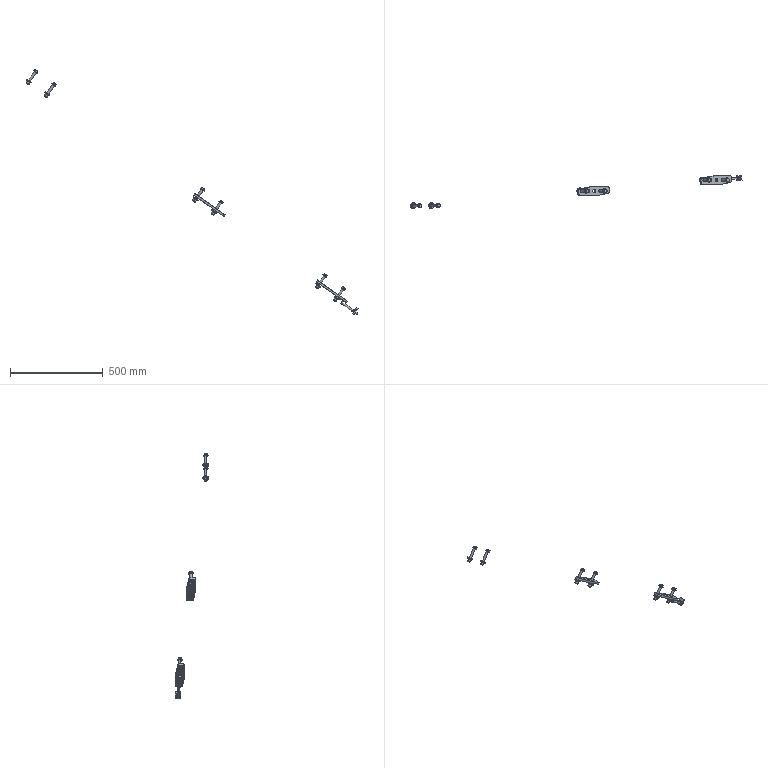Part | STEP file | COMPOUND | 36 solids | 304 faces | box 1791 x 180.745 x 1321 mm | volume 266287 mm3 | plane 191 | cylinder 73 | cone 39 | torus 1 | commonest cylinder face diameters 13 x13 20 x12 18 x8 24 x7 12 x6 12.001 x6